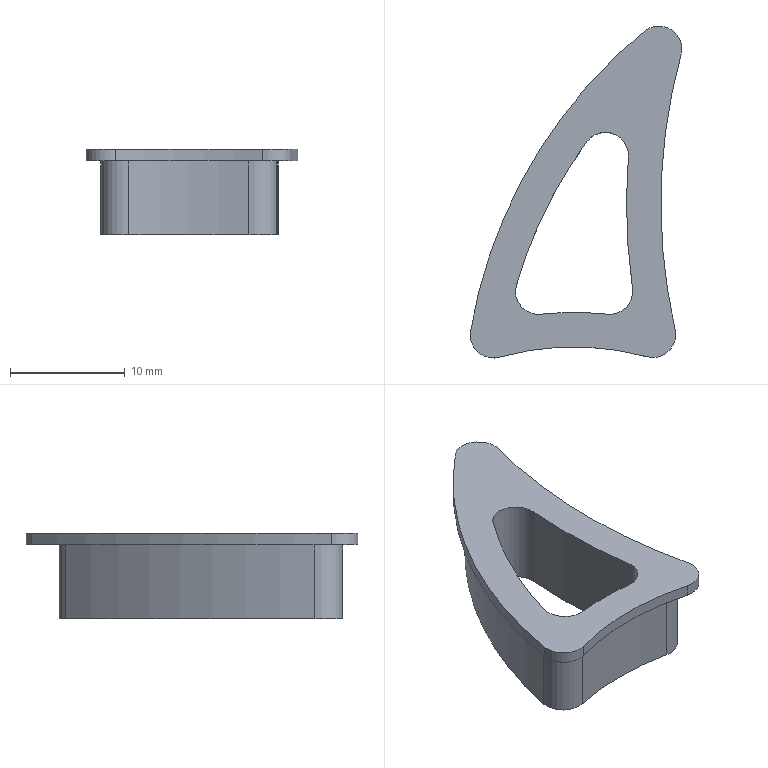Part | NX | features DATUM_CSYS 4, EXTRUDE 3, SKETCH 3, BLEND 1, CPROJ 1 | 1 solid | 21 faces | box 18.409 x 28.891 x 7.4 mm | volume 1102 mm3 | cylinder 18 | plane 3 | commonest cylinder face diameters 4 x9 48 x1 50 x1 54 x1 80 x1 84 x1
STEP:
#1=CARTESIAN_POINT('',(-5.33,24.506,0.));
#2=VERTEX_POINT('',#1);
#3=CARTESIAN_POINT('',(5.135,24.548,0.));
#4=VERTEX_POINT('',#3);
#5=CARTESIAN_POINT('',(0.,0.0809,0.));
#6=DIRECTION('',(0.,0.,-1.));
#7=DIRECTION('',(1.,0.,0.));
#8=AXIS2_PLACEMENT_3D('',#5,#6,#7);
#9=CIRCLE('',#8,25.);
#10=EDGE_CURVE('',#2,#4,#9,.T.);
#11=ORIENTED_EDGE('',*,*,#10,.F.);
#12=CARTESIAN_POINT('',(-7.715,26.867,0.));
#13=VERTEX_POINT('',#12);
#14=CARTESIAN_POINT('',(-5.757,26.46,0.));
#15=DIRECTION('',(0.,0.,-1.));
#16=DIRECTION('',(-1.,0.,0.));
#17=AXIS2_PLACEMENT_3D('',#14,#15,#16);
#18=CIRCLE('',#17,2.);
#19=EDGE_CURVE('',#2,#13,#18,.T.);
#20=ORIENTED_EDGE('',*,*,#19,.T.);
#21=CARTESIAN_POINT('',(4.276,48.579,0.));
#22=VERTEX_POINT('',#21);
#23=CARTESIAN_POINT('',(33.407,18.323,0.));
#24=DIRECTION('',(0.,0.,1.));
#25=DIRECTION('',(1.,0.,0.));
#26=AXIS2_PLACEMENT_3D('',#23,#24,#25);
#27=CIRCLE('',#26,42.);
#28=EDGE_CURVE('',#22,#13,#27,.T.);
#29=ORIENTED_EDGE('',*,*,#28,.F.);
#30=CARTESIAN_POINT('',(7.621,46.73,0.));
#31=VERTEX_POINT('',#30);
#32=CARTESIAN_POINT('',(5.663,47.138,0.));
#33=DIRECTION('',(0.,0.,-1.));
#34=DIRECTION('',(-1.,0.,0.));
#35=AXIS2_PLACEMENT_3D('',#32,#33,#34);
#36=CIRCLE('',#35,2.);
#37=EDGE_CURVE('',#22,#31,#36,.T.);
#38=ORIENTED_EDGE('',*,*,#37,.T.);
#39=CARTESIAN_POINT('',(7.509,26.891,0.));
#40=VERTEX_POINT('',#39);
#41=CARTESIAN_POINT('',(56.57,36.531,0.));
#42=DIRECTION('',(0.,0.,-1.));
#43=DIRECTION('',(1.,0.,0.));
#44=AXIS2_PLACEMENT_3D('',#41,#42,#43);
#45=CIRCLE('',#44,50.);
#46=EDGE_CURVE('',#40,#31,#45,.T.);
#47=ORIENTED_EDGE('',*,*,#46,.F.);
#48=CARTESIAN_POINT('',(5.546,26.505,0.));
#49=DIRECTION('',(0.,0.,-1.));
#50=DIRECTION('',(-1.,0.,0.));
#51=AXIS2_PLACEMENT_3D('',#48,#49,#50);
#52=CIRCLE('',#51,2.);
#53=EDGE_CURVE('',#40,#4,#52,.T.);
#54=ORIENTED_EDGE('',*,*,#53,.T.);
#55=EDGE_LOOP('',(#11,#20,#29,#38,#47,#54));
#56=FACE_BOUND('',#55,.T.);
#57=CARTESIAN_POINT('',(-2.874,26.928,0.));
#58=VERTEX_POINT('',#57);
#59=CARTESIAN_POINT('',(-5.007,29.474,0.));
#60=VERTEX_POINT('',#59);
#61=CARTESIAN_POINT('',(-3.087,28.916,0.));
#62=DIRECTION('',(0.,0.,-1.));
#63=DIRECTION('',(1.,0.,0.));
#64=AXIS2_PLACEMENT_3D('',#61,#62,#63);
#65=CIRCLE('',#64,2.);
#66=EDGE_CURVE('',#58,#60,#65,.T.);
#67=ORIENTED_EDGE('',*,*,#66,.F.);
#68=CARTESIAN_POINT('',(2.896,26.925,0.));
#69=VERTEX_POINT('',#68);
#70=CARTESIAN_POINT('',(0.,0.0809,0.));
#71=DIRECTION('',(0.,0.,1.));
#72=DIRECTION('',(1.,0.,0.));
#73=AXIS2_PLACEMENT_3D('',#70,#71,#72);
#74=CIRCLE('',#73,27.);
#75=EDGE_CURVE('',#69,#58,#74,.T.);
#76=ORIENTED_EDGE('',*,*,#75,.F.);
#77=CARTESIAN_POINT('',(5.09,29.196,0.));
#78=VERTEX_POINT('',#77);
#79=CARTESIAN_POINT('',(3.11,28.914,0.));
#80=DIRECTION('',(0.,0.,-1.));
#81=DIRECTION('',(1.,0.,0.));
#82=AXIS2_PLACEMENT_3D('',#79,#80,#81);
#83=CIRCLE('',#82,2.);
#84=EDGE_CURVE('',#78,#69,#83,.T.);
#85=ORIENTED_EDGE('',*,*,#84,.F.);
#86=CARTESIAN_POINT('',(4.73,40.6,0.));
#87=VERTEX_POINT('',#86);
#88=CARTESIAN_POINT('',(56.57,36.531,0.));
#89=DIRECTION('',(0.,0.,1.));
#90=DIRECTION('',(1.,0.,0.));
#91=AXIS2_PLACEMENT_3D('',#88,#89,#90);
#92=CIRCLE('',#91,52.);
#93=EDGE_CURVE('',#87,#78,#92,.T.);
#94=ORIENTED_EDGE('',*,*,#93,.F.);
#95=CARTESIAN_POINT('',(1.122,41.938,0.));
#96=VERTEX_POINT('',#95);
#97=CARTESIAN_POINT('',(2.736,40.757,0.));
#98=DIRECTION('',(0.,0.,-1.));
#99=DIRECTION('',(1.,0.,0.));
#100=AXIS2_PLACEMENT_3D('',#97,#98,#99);
#101=CIRCLE('',#100,2.);
#102=EDGE_CURVE('',#96,#87,#101,.T.);
#103=ORIENTED_EDGE('',*,*,#102,.F.);
#104=CARTESIAN_POINT('',(33.407,18.323,0.));
#105=DIRECTION('',(0.,0.,-1.));
#106=DIRECTION('',(1.,0.,0.));
#107=AXIS2_PLACEMENT_3D('',#104,#105,#106);
#108=CIRCLE('',#107,40.);
#109=EDGE_CURVE('',#60,#96,#108,.T.);
#110=ORIENTED_EDGE('',*,*,#109,.F.);
#111=EDGE_LOOP('',(#67,#76,#85,#94,#103,#110));
#112=FACE_BOUND('',#111,.T.);
#113=CARTESIAN_POINT('',(28.285,18.306,0.));
#114=DIRECTION('',(0.,0.,-1.));
#115=DIRECTION('',(-1.,0.,0.));
#116=AXIS2_PLACEMENT_3D('',#113,#114,#115);
#117=PLANE('',#116);
#118=ADVANCED_FACE('',(#56,#112),#117,.T.);
#119=CARTESIAN_POINT('',(-8.999,25.445,7.4));
#120=VERTEX_POINT('',#119);
#121=CARTESIAN_POINT('',(6.113,51.55,7.4));
#122=VERTEX_POINT('',#121);
#123=CARTESIAN_POINT('',(33.407,18.323,7.4));
#124=DIRECTION('',(0.,0.,1.));
#125=DIRECTION('',(1.,0.,0.));
#126=AXIS2_PLACEMENT_3D('',#123,#124,#125);
#127=CIRCLE('',#126,43.);
#128=EDGE_CURVE('',#120,#122,#127,.F.);
#129=ORIENTED_EDGE('',*,*,#128,.F.);
#130=CARTESIAN_POINT('',(-6.486,23.188,7.4));
#131=VERTEX_POINT('',#130);
#132=CARTESIAN_POINT('',(-7.027,25.113,7.4));
#133=DIRECTION('',(0.,0.,-1.));
#134=DIRECTION('',(-1.,0.,0.));
#135=AXIS2_PLACEMENT_3D('',#132,#133,#134);
#136=CIRCLE('',#135,2.);
#137=EDGE_CURVE('',#120,#131,#136,.F.);
#138=ORIENTED_EDGE('',*,*,#137,.T.);
#139=CARTESIAN_POINT('',(6.327,23.232,7.4));
#140=VERTEX_POINT('',#139);
#141=CARTESIAN_POINT('',(0.,0.0809,7.4));
#142=DIRECTION('',(0.,0.,-1.));
#143=DIRECTION('',(1.,0.,0.));
#144=AXIS2_PLACEMENT_3D('',#141,#142,#143);
#145=CIRCLE('',#144,24.);
#146=EDGE_CURVE('',#140,#131,#145,.F.);
#147=ORIENTED_EDGE('',*,*,#146,.F.);
#148=CARTESIAN_POINT('',(8.804,25.607,7.4));
#149=VERTEX_POINT('',#148);
#150=CARTESIAN_POINT('',(6.854,25.161,7.4));
#151=DIRECTION('',(0.,0.,-1.));
#152=DIRECTION('',(-1.,0.,0.));
#153=AXIS2_PLACEMENT_3D('',#150,#151,#152);
#154=CIRCLE('',#153,2.);
#155=EDGE_CURVE('',#140,#149,#154,.F.);
#156=ORIENTED_EDGE('',*,*,#155,.T.);
#157=CARTESIAN_POINT('',(9.311,49.476,7.4));
#158=VERTEX_POINT('',#157);
#159=CARTESIAN_POINT('',(56.57,36.531,7.4));
#160=DIRECTION('',(0.,0.,-1.));
#161=DIRECTION('',(1.,0.,0.));
#162=AXIS2_PLACEMENT_3D('',#159,#160,#161);
#163=CIRCLE('',#162,49.);
#164=EDGE_CURVE('',#158,#149,#163,.F.);
#165=ORIENTED_EDGE('',*,*,#164,.F.);
#166=CARTESIAN_POINT('',(7.382,50.004,7.4));
#167=DIRECTION('',(0.,0.,-1.));
#168=DIRECTION('',(-1.,0.,0.));
#169=AXIS2_PLACEMENT_3D('',#166,#167,#168);
#170=CIRCLE('',#169,2.);
#171=EDGE_CURVE('',#158,#122,#170,.F.);
#172=ORIENTED_EDGE('',*,*,#171,.T.);
#173=EDGE_LOOP('',(#129,#138,#147,#156,#165,#172));
#174=FACE_BOUND('',#173,.T.);
#175=CARTESIAN_POINT('',(2.896,26.925,7.4));
#176=VERTEX_POINT('',#175);
#177=CARTESIAN_POINT('',(-2.874,26.928,7.4));
#178=VERTEX_POINT('',#177);
#179=CARTESIAN_POINT('',(0.,0.0809,7.4));
#180=DIRECTION('',(0.,0.,-1.));
#181=DIRECTION('',(-1.,0.,0.));
#182=AXIS2_PLACEMENT_3D('',#179,#180,#181);
#183=CIRCLE('',#182,27.);
#184=EDGE_CURVE('',#176,#178,#183,.F.);
#185=ORIENTED_EDGE('',*,*,#184,.T.);
#186=CARTESIAN_POINT('',(-5.007,29.474,7.4));
#187=VERTEX_POINT('',#186);
#188=CARTESIAN_POINT('',(-3.087,28.916,7.4));
#189=DIRECTION('',(0.,0.,-1.));
#190=DIRECTION('',(-1.,0.,0.));
#191=AXIS2_PLACEMENT_3D('',#188,#189,#190);
#192=CIRCLE('',#191,2.);
#193=EDGE_CURVE('',#178,#187,#192,.T.);
#194=ORIENTED_EDGE('',*,*,#193,.T.);
#195=CARTESIAN_POINT('',(1.122,41.938,7.4));
#196=VERTEX_POINT('',#195);
#197=CARTESIAN_POINT('',(33.407,18.323,7.4));
#198=DIRECTION('',(0.,0.,-1.));
#199=DIRECTION('',(-1.,0.,0.));
#200=AXIS2_PLACEMENT_3D('',#197,#198,#199);
#201=CIRCLE('',#200,40.);
#202=EDGE_CURVE('',#187,#196,#201,.T.);
#203=ORIENTED_EDGE('',*,*,#202,.T.);
#204=CARTESIAN_POINT('',(4.73,40.6,7.4));
#205=VERTEX_POINT('',#204);
#206=CARTESIAN_POINT('',(2.736,40.757,7.4));
#207=DIRECTION('',(0.,0.,-1.));
#208=DIRECTION('',(-1.,0.,0.));
#209=AXIS2_PLACEMENT_3D('',#206,#207,#208);
#210=CIRCLE('',#209,2.);
#211=EDGE_CURVE('',#196,#205,#210,.T.);
#212=ORIENTED_EDGE('',*,*,#211,.T.);
#213=CARTESIAN_POINT('',(5.09,29.196,7.4));
#214=VERTEX_POINT('',#213);
#215=CARTESIAN_POINT('',(56.57,36.531,7.4));
#216=DIRECTION('',(0.,0.,-1.));
#217=DIRECTION('',(-1.,0.,0.));
#218=AXIS2_PLACEMENT_3D('',#215,#216,#217);
#219=CIRCLE('',#218,52.);
#220=EDGE_CURVE('',#205,#214,#219,.F.);
#221=ORIENTED_EDGE('',*,*,#220,.T.);
#222=CARTESIAN_POINT('',(3.11,28.914,7.4));
#223=DIRECTION('',(0.,0.,-1.));
#224=DIRECTION('',(-1.,0.,0.));
#225=AXIS2_PLACEMENT_3D('',#222,#223,#224);
#226=CIRCLE('',#225,2.);
#227=EDGE_CURVE('',#214,#176,#226,.T.);
#228=ORIENTED_EDGE('',*,*,#227,.T.);
#229=EDGE_LOOP('',(#185,#194,#203,#212,#221,#228));
#230=FACE_BOUND('',#229,.T.);
#231=CARTESIAN_POINT('',(28.285,18.306,7.4));
#232=DIRECTION('',(0.,0.,-1.));
#233=DIRECTION('',(-1.,0.,0.));
#234=AXIS2_PLACEMENT_3D('',#231,#232,#233);
#235=PLANE('',#234);
#236=ADVANCED_FACE('',(#174,#230),#235,.F.);
#237=CARTESIAN_POINT('',(-5.33,24.506,6.4));
#238=VERTEX_POINT('',#237);
#239=CARTESIAN_POINT('',(5.135,24.548,6.4));
#240=VERTEX_POINT('',#239);
#241=CARTESIAN_POINT('',(0.,0.0809,6.4));
#242=DIRECTION('',(0.,0.,1.));
#243=DIRECTION('',(1.,0.,0.));
#244=AXIS2_PLACEMENT_3D('',#241,#242,#243);
#245=CIRCLE('',#244,25.);
#246=EDGE_CURVE('',#238,#240,#245,.F.);
#247=ORIENTED_EDGE('',*,*,#246,.F.);
#248=CARTESIAN_POINT('',(-5.33,24.506,7.4));
#249=DIRECTION('',(0.,0.,-1.));
#250=VECTOR('',#249,1000.);
#251=LINE('',#248,#250);
#252=EDGE_CURVE('',#238,#2,#251,.T.);
#253=ORIENTED_EDGE('',*,*,#252,.T.);
#254=ORIENTED_EDGE('',*,*,#10,.T.);
#255=CARTESIAN_POINT('',(5.135,24.548,7.4));
#256=DIRECTION('',(0.,0.,-1.));
#257=VECTOR('',#256,1000.);
#258=LINE('',#255,#257);
#259=EDGE_CURVE('',#4,#240,#258,.F.);
#260=ORIENTED_EDGE('',*,*,#259,.T.);
#261=EDGE_LOOP('',(#247,#253,#254,#260));
#262=FACE_BOUND('',#261,.T.);
#263=CARTESIAN_POINT('',(0.,0.0809,7.4));
#264=DIRECTION('',(0.,0.,-1.));
#265=DIRECTION('',(-1.,0.,0.));
#266=AXIS2_PLACEMENT_3D('',#263,#264,#265);
#267=CYLINDRICAL_SURFACE('',#266,25.);
#268=ADVANCED_FACE('',(#262),#267,.F.);
#269=CARTESIAN_POINT('',(7.509,26.891,6.4));
#270=VERTEX_POINT('',#269);
#271=CARTESIAN_POINT('',(7.621,46.73,6.4));
#272=VERTEX_POINT('',#271);
#273=CARTESIAN_POINT('',(56.57,36.531,6.4));
#274=DIRECTION('',(0.,0.,1.));
#275=DIRECTION('',(1.,0.,0.));
#276=AXIS2_PLACEMENT_3D('',#273,#274,#275);
#277=CIRCLE('',#276,50.);
#278=EDGE_CURVE('',#270,#272,#277,.F.);
#279=ORIENTED_EDGE('',*,*,#278,.F.);
#280=CARTESIAN_POINT('',(7.509,26.891,7.4));
#281=DIRECTION('',(0.,0.,-1.));
#282=VECTOR('',#281,1000.);
#283=LINE('',#280,#282);
#284=EDGE_CURVE('',#270,#40,#283,.T.);
#285=ORIENTED_EDGE('',*,*,#284,.T.);
#286=ORIENTED_EDGE('',*,*,#46,.T.);
#287=CARTESIAN_POINT('',(7.621,46.73,7.4));
#288=DIRECTION('',(0.,0.,-1.));
#289=VECTOR('',#288,1000.);
#290=LINE('',#287,#289);
#291=EDGE_CURVE('',#31,#272,#290,.F.);
#292=ORIENTED_EDGE('',*,*,#291,.T.);
#293=EDGE_LOOP('',(#279,#285,#286,#292));
#294=FACE_BOUND('',#293,.T.);
#295=CARTESIAN_POINT('',(56.57,36.531,7.4));
#296=DIRECTION('',(0.,0.,-1.));
#297=DIRECTION('',(-1.,0.,0.));
#298=AXIS2_PLACEMENT_3D('',#295,#296,#297);
#299=CYLINDRICAL_SURFACE('',#298,50.);
#300=ADVANCED_FACE('',(#294),#299,.F.);
#301=ORIENTED_EDGE('',*,*,#28,.T.);
#302=CARTESIAN_POINT('',(-7.715,26.867,6.4));
#303=VERTEX_POINT('',#302);
#304=CARTESIAN_POINT('',(-7.715,26.867,7.4));
#305=DIRECTION('',(0.,0.,-1.));
#306=VECTOR('',#305,1000.);
#307=LINE('',#304,#306);
#308=EDGE_CURVE('',#13,#303,#307,.F.);
#309=ORIENTED_EDGE('',*,*,#308,.T.);
#310=CARTESIAN_POINT('',(4.276,48.579,6.4));
#311=VERTEX_POINT('',#310);
#312=CARTESIAN_POINT('',(33.407,18.323,6.4));
#313=DIRECTION('',(0.,0.,-1.));
#314=DIRECTION('',(1.,0.,0.));
#315=AXIS2_PLACEMENT_3D('',#312,#313,#314);
#316=CIRCLE('',#315,42.);
#317=EDGE_CURVE('',#311,#303,#316,.F.);
#318=ORIENTED_EDGE('',*,*,#317,.F.);
#319=CARTESIAN_POINT('',(4.276,48.579,7.4));
#320=DIRECTION('',(0.,0.,-1.));
#321=VECTOR('',#320,1000.);
#322=LINE('',#319,#321);
#323=EDGE_CURVE('',#311,#22,#322,.T.);
#324=ORIENTED_EDGE('',*,*,#323,.T.);
#325=EDGE_LOOP('',(#301,#309,#318,#324));
#326=FACE_BOUND('',#325,.T.);
#327=CARTESIAN_POINT('',(33.407,18.323,7.4));
#328=DIRECTION('',(0.,0.,-1.));
#329=DIRECTION('',(-1.,0.,0.));
#330=AXIS2_PLACEMENT_3D('',#327,#328,#329);
#331=CYLINDRICAL_SURFACE('',#330,42.);
#332=ADVANCED_FACE('',(#326),#331,.T.);
#333=ORIENTED_EDGE('',*,*,#146,.T.);
#334=CARTESIAN_POINT('',(-6.486,23.188,6.4));
#335=VERTEX_POINT('',#334);
#336=CARTESIAN_POINT('',(-6.486,23.188,6.4));
#337=DIRECTION('',(0.,0.,1.));
#338=VECTOR('',#337,1000.);
#339=LINE('',#336,#338);
#340=EDGE_CURVE('',#131,#335,#339,.F.);
#341=ORIENTED_EDGE('',*,*,#340,.T.);
#342=CARTESIAN_POINT('',(6.327,23.232,6.4));
#343=VERTEX_POINT('',#342);
#344=CARTESIAN_POINT('',(0.,0.0809,6.4));
#345=DIRECTION('',(0.,0.,-1.));
#346=DIRECTION('',(1.,0.,0.));
#347=AXIS2_PLACEMENT_3D('',#344,#345,#346);
#348=CIRCLE('',#347,24.);
#349=EDGE_CURVE('',#343,#335,#348,.F.);
#350=ORIENTED_EDGE('',*,*,#349,.F.);
#351=CARTESIAN_POINT('',(6.327,23.232,6.4));
#352=DIRECTION('',(0.,0.,1.));
#353=VECTOR('',#352,1000.);
#354=LINE('',#351,#353);
#355=EDGE_CURVE('',#343,#140,#354,.T.);
#356=ORIENTED_EDGE('',*,*,#355,.T.);
#357=EDGE_LOOP('',(#333,#341,#350,#356));
#358=FACE_BOUND('',#357,.T.);
#359=CARTESIAN_POINT('',(0.,0.0809,6.4));
#360=DIRECTION('',(0.,0.,1.));
#361=DIRECTION('',(1.,0.,0.));
#362=AXIS2_PLACEMENT_3D('',#359,#360,#361);
#363=CYLINDRICAL_SURFACE('',#362,24.);
#364=ADVANCED_FACE('',(#358),#363,.F.);
#365=ORIENTED_EDGE('',*,*,#164,.T.);
#366=CARTESIAN_POINT('',(8.804,25.607,6.4));
#367=VERTEX_POINT('',#366);
#368=CARTESIAN_POINT('',(8.804,25.607,6.4));
#369=DIRECTION('',(0.,0.,1.));
#370=VECTOR('',#369,1000.);
#371=LINE('',#368,#370);
#372=EDGE_CURVE('',#149,#367,#371,.F.);
#373=ORIENTED_EDGE('',*,*,#372,.T.);
#374=CARTESIAN_POINT('',(9.311,49.476,6.4));
#375=VERTEX_POINT('',#374);
#376=CARTESIAN_POINT('',(56.57,36.531,6.4));
#377=DIRECTION('',(0.,0.,-1.));
#378=DIRECTION('',(1.,0.,0.));
#379=AXIS2_PLACEMENT_3D('',#376,#377,#378);
#380=CIRCLE('',#379,49.);
#381=EDGE_CURVE('',#375,#367,#380,.F.);
#382=ORIENTED_EDGE('',*,*,#381,.F.);
#383=CARTESIAN_POINT('',(9.311,49.476,6.4));
#384=DIRECTION('',(0.,0.,1.));
#385=VECTOR('',#384,1000.);
#386=LINE('',#383,#385);
#387=EDGE_CURVE('',#375,#158,#386,.T.);
#388=ORIENTED_EDGE('',*,*,#387,.T.);
#389=EDGE_LOOP('',(#365,#373,#382,#388));
#390=FACE_BOUND('',#389,.T.);
#391=CARTESIAN_POINT('',(56.57,36.531,6.4));
#392=DIRECTION('',(0.,0.,1.));
#393=DIRECTION('',(1.,0.,0.));
#394=AXIS2_PLACEMENT_3D('',#391,#392,#393);
#395=CYLINDRICAL_SURFACE('',#394,49.);
#396=ADVANCED_FACE('',(#390),#395,.F.);
#397=CARTESIAN_POINT('',(-8.999,25.445,6.4));
#398=VERTEX_POINT('',#397);
#399=CARTESIAN_POINT('',(6.113,51.55,6.4));
#400=VERTEX_POINT('',#399);
#401=CARTESIAN_POINT('',(33.407,18.323,6.4));
#402=DIRECTION('',(0.,0.,1.));
#403=DIRECTION('',(1.,0.,0.));
#404=AXIS2_PLACEMENT_3D('',#401,#402,#403);
#405=CIRCLE('',#404,43.);
#406=EDGE_CURVE('',#398,#400,#405,.F.);
#407=ORIENTED_EDGE('',*,*,#406,.F.);
#408=CARTESIAN_POINT('',(-8.999,25.445,6.4));
#409=DIRECTION('',(0.,0.,1.));
#410=VECTOR('',#409,1000.);
#411=LINE('',#408,#410);
#412=EDGE_CURVE('',#398,#120,#411,.T.);
#413=ORIENTED_EDGE('',*,*,#412,.T.);
#414=ORIENTED_EDGE('',*,*,#128,.T.);
#415=CARTESIAN_POINT('',(6.113,51.55,6.4));
#416=DIRECTION('',(0.,0.,1.));
#417=VECTOR('',#416,1000.);
#418=LINE('',#415,#417);
#419=EDGE_CURVE('',#122,#400,#418,.F.);
#420=ORIENTED_EDGE('',*,*,#419,.T.);
#421=EDGE_LOOP('',(#407,#413,#414,#420));
#422=FACE_BOUND('',#421,.T.);
#423=CARTESIAN_POINT('',(33.407,18.323,6.4));
#424=DIRECTION('',(0.,0.,1.));
#425=DIRECTION('',(1.,0.,0.));
#426=AXIS2_PLACEMENT_3D('',#423,#424,#425);
#427=CYLINDRICAL_SURFACE('',#426,43.);
#428=ADVANCED_FACE('',(#422),#427,.T.);
#429=ORIENTED_EDGE('',*,*,#381,.T.);
#430=CARTESIAN_POINT('',(6.854,25.161,6.4));
#431=DIRECTION('',(0.,0.,-1.));
#432=DIRECTION('',(-1.,0.,0.));
#433=AXIS2_PLACEMENT_3D('',#430,#431,#432);
#434=CIRCLE('',#433,2.);
#435=EDGE_CURVE('',#367,#343,#434,.T.);
#436=ORIENTED_EDGE('',*,*,#435,.T.);
#437=ORIENTED_EDGE('',*,*,#349,.T.);
#438=CARTESIAN_POINT('',(-7.027,25.113,6.4));
#439=DIRECTION('',(0.,0.,-1.));
#440=DIRECTION('',(-1.,0.,0.));
#441=AXIS2_PLACEMENT_3D('',#438,#439,#440);
#442=CIRCLE('',#441,2.);
#443=EDGE_CURVE('',#335,#398,#442,.T.);
#444=ORIENTED_EDGE('',*,*,#443,.T.);
#445=ORIENTED_EDGE('',*,*,#406,.T.);
#446=CARTESIAN_POINT('',(7.382,50.004,6.4));
#447=DIRECTION('',(0.,0.,-1.));
#448=DIRECTION('',(-1.,0.,0.));
#449=AXIS2_PLACEMENT_3D('',#446,#447,#448);
#450=CIRCLE('',#449,2.);
#451=EDGE_CURVE('',#400,#375,#450,.T.);
#452=ORIENTED_EDGE('',*,*,#451,.T.);
#453=EDGE_LOOP('',(#429,#436,#437,#444,#445,#452));
#454=FACE_BOUND('',#453,.T.);
#455=ORIENTED_EDGE('',*,*,#317,.T.);
#456=CARTESIAN_POINT('',(-5.757,26.46,6.4));
#457=DIRECTION('',(0.,0.,-1.));
#458=DIRECTION('',(-1.,0.,0.));
#459=AXIS2_PLACEMENT_3D('',#456,#457,#458);
#460=CIRCLE('',#459,2.);
#461=EDGE_CURVE('',#303,#238,#460,.F.);
#462=ORIENTED_EDGE('',*,*,#461,.T.);
#463=ORIENTED_EDGE('',*,*,#246,.T.);
#464=CARTESIAN_POINT('',(5.546,26.505,6.4));
#465=DIRECTION('',(0.,0.,-1.));
#466=DIRECTION('',(-1.,0.,0.));
#467=AXIS2_PLACEMENT_3D('',#464,#465,#466);
#468=CIRCLE('',#467,2.);
#469=EDGE_CURVE('',#240,#270,#468,.F.);
#470=ORIENTED_EDGE('',*,*,#469,.T.);
#471=ORIENTED_EDGE('',*,*,#278,.T.);
#472=CARTESIAN_POINT('',(5.663,47.138,6.4));
#473=DIRECTION('',(0.,0.,-1.));
#474=DIRECTION('',(-1.,0.,0.));
#475=AXIS2_PLACEMENT_3D('',#472,#473,#474);
#476=CIRCLE('',#475,2.);
#477=EDGE_CURVE('',#272,#311,#476,.F.);
#478=ORIENTED_EDGE('',*,*,#477,.T.);
#479=EDGE_LOOP('',(#455,#462,#463,#470,#471,#478));
#480=FACE_BOUND('',#479,.T.);
#481=CARTESIAN_POINT('',(28.285,18.306,6.4));
#482=DIRECTION('',(0.,0.,-1.));
#483=DIRECTION('',(-1.,0.,0.));
#484=AXIS2_PLACEMENT_3D('',#481,#482,#483);
#485=PLANE('',#484);
#486=ADVANCED_FACE('',(#454,#480),#485,.T.);
#487=CARTESIAN_POINT('',(-2.874,26.928,55000.));
#488=DIRECTION('',(0.,0.,-1.));
#489=VECTOR('',#488,1000.);
#490=LINE('',#487,#489);
#491=EDGE_CURVE('',#58,#178,#490,.F.);
#492=ORIENTED_EDGE('',*,*,#491,.F.);
#493=ORIENTED_EDGE('',*,*,#66,.T.);
#494=CARTESIAN_POINT('',(-5.007,29.474,55000.));
#495=DIRECTION('',(0.,0.,-1.));
#496=VECTOR('',#495,1000.);
#497=LINE('',#494,#496);
#498=EDGE_CURVE('',#60,#187,#497,.F.);
#499=ORIENTED_EDGE('',*,*,#498,.T.);
#500=ORIENTED_EDGE('',*,*,#193,.F.);
#501=EDGE_LOOP('',(#492,#493,#499,#500));
#502=FACE_BOUND('',#501,.T.);
#503=CARTESIAN_POINT('',(-3.087,28.916,55000.));
#504=DIRECTION('',(0.,0.,-1.));
#505=DIRECTION('',(-1.,0.,0.));
#506=AXIS2_PLACEMENT_3D('',#503,#504,#505);
#507=CYLINDRICAL_SURFACE('',#506,2.);
#508=ADVANCED_FACE('',(#502),#507,.F.);
#509=ORIENTED_EDGE('',*,*,#498,.F.);
#510=ORIENTED_EDGE('',*,*,#109,.T.);
#511=CARTESIAN_POINT('',(1.122,41.938,55000.));
#512=DIRECTION('',(0.,0.,-1.));
#513=VECTOR('',#512,1000.);
#514=LINE('',#511,#513);
#515=EDGE_CURVE('',#96,#196,#514,.F.);
#516=ORIENTED_EDGE('',*,*,#515,.T.);
#517=ORIENTED_EDGE('',*,*,#202,.F.);
#518=EDGE_LOOP('',(#509,#510,#516,#517));
#519=FACE_BOUND('',#518,.T.);
#520=CARTESIAN_POINT('',(33.407,18.323,55000.));
#521=DIRECTION('',(0.,0.,-1.));
#522=DIRECTION('',(-1.,0.,0.));
#523=AXIS2_PLACEMENT_3D('',#520,#521,#522);
#524=CYLINDRICAL_SURFACE('',#523,40.);
#525=ADVANCED_FACE('',(#519),#524,.F.);
#526=ORIENTED_EDGE('',*,*,#515,.F.);
#527=ORIENTED_EDGE('',*,*,#102,.T.);
#528=CARTESIAN_POINT('',(4.73,40.6,55000.));
#529=DIRECTION('',(0.,0.,-1.));
#530=VECTOR('',#529,1000.);
#531=LINE('',#528,#530);
#532=EDGE_CURVE('',#87,#205,#531,.F.);
#533=ORIENTED_EDGE('',*,*,#532,.T.);
#534=ORIENTED_EDGE('',*,*,#211,.F.);
#535=EDGE_LOOP('',(#526,#527,#533,#534));
#536=FACE_BOUND('',#535,.T.);
#537=CARTESIAN_POINT('',(2.736,40.757,55000.));
#538=DIRECTION('',(0.,0.,-1.));
#539=DIRECTION('',(-1.,0.,0.));
#540=AXIS2_PLACEMENT_3D('',#537,#538,#539);
#541=CYLINDRICAL_SURFACE('',#540,2.);
#542=ADVANCED_FACE('',(#536),#541,.F.);
#543=ORIENTED_EDGE('',*,*,#532,.F.);
#544=ORIENTED_EDGE('',*,*,#93,.T.);
#545=CARTESIAN_POINT('',(5.09,29.196,55000.));
#546=DIRECTION('',(0.,0.,-1.));
#547=VECTOR('',#546,1000.);
#548=LINE('',#545,#547);
#549=EDGE_CURVE('',#78,#214,#548,.F.);
#550=ORIENTED_EDGE('',*,*,#549,.T.);
#551=ORIENTED_EDGE('',*,*,#220,.F.);
#552=EDGE_LOOP('',(#543,#544,#550,#551));
#553=FACE_BOUND('',#552,.T.);
#554=CARTESIAN_POINT('',(56.57,36.531,55000.));
#555=DIRECTION('',(0.,0.,-1.));
#556=DIRECTION('',(-1.,0.,0.));
#557=AXIS2_PLACEMENT_3D('',#554,#555,#556);
#558=CYLINDRICAL_SURFACE('',#557,52.);
#559=ADVANCED_FACE('',(#553),#558,.T.);
#560=ORIENTED_EDGE('',*,*,#549,.F.);
#561=ORIENTED_EDGE('',*,*,#84,.T.);
#562=CARTESIAN_POINT('',(2.896,26.925,55000.));
#563=DIRECTION('',(0.,0.,-1.));
#564=VECTOR('',#563,1000.);
#565=LINE('',#562,#564);
#566=EDGE_CURVE('',#69,#176,#565,.F.);
#567=ORIENTED_EDGE('',*,*,#566,.T.);
#568=ORIENTED_EDGE('',*,*,#227,.F.);
#569=EDGE_LOOP('',(#560,#561,#567,#568));
#570=FACE_BOUND('',#569,.T.);
#571=CARTESIAN_POINT('',(3.11,28.914,55000.));
#572=DIRECTION('',(0.,0.,-1.));
#573=DIRECTION('',(-1.,0.,0.));
#574=AXIS2_PLACEMENT_3D('',#571,#572,#573);
#575=CYLINDRICAL_SURFACE('',#574,2.);
#576=ADVANCED_FACE('',(#570),#575,.F.);
#577=ORIENTED_EDGE('',*,*,#566,.F.);
#578=ORIENTED_EDGE('',*,*,#75,.T.);
#579=ORIENTED_EDGE('',*,*,#491,.T.);
#580=ORIENTED_EDGE('',*,*,#184,.F.);
#581=EDGE_LOOP('',(#577,#578,#579,#580));
#582=FACE_BOUND('',#581,.T.);
#583=CARTESIAN_POINT('',(0.,0.0809,55000.));
#584=DIRECTION('',(0.,0.,-1.));
#585=DIRECTION('',(-1.,0.,0.));
#586=AXIS2_PLACEMENT_3D('',#583,#584,#585);
#587=CYLINDRICAL_SURFACE('',#586,27.);
#588=ADVANCED_FACE('',(#582),#587,.T.);
#589=ORIENTED_EDGE('',*,*,#137,.F.);
#590=ORIENTED_EDGE('',*,*,#412,.F.);
#591=ORIENTED_EDGE('',*,*,#443,.F.);
#592=ORIENTED_EDGE('',*,*,#340,.F.);
#593=EDGE_LOOP('',(#589,#590,#591,#592));
#594=FACE_BOUND('',#593,.T.);
#595=CARTESIAN_POINT('',(-7.027,25.113,6.4));
#596=DIRECTION('',(0.,0.,1.));
#597=DIRECTION('',(1.,0.,0.));
#598=AXIS2_PLACEMENT_3D('',#595,#596,#597);
#599=CYLINDRICAL_SURFACE('',#598,2.);
#600=ADVANCED_FACE('',(#594),#599,.T.);
#601=ORIENTED_EDGE('',*,*,#155,.F.);
#602=ORIENTED_EDGE('',*,*,#355,.F.);
#603=ORIENTED_EDGE('',*,*,#435,.F.);
#604=ORIENTED_EDGE('',*,*,#372,.F.);
#605=EDGE_LOOP('',(#601,#602,#603,#604));
#606=FACE_BOUND('',#605,.T.);
#607=CARTESIAN_POINT('',(6.854,25.161,6.4));
#608=DIRECTION('',(0.,0.,-1.));
#609=DIRECTION('',(-1.,0.,0.));
#610=AXIS2_PLACEMENT_3D('',#607,#608,#609);
#611=CYLINDRICAL_SURFACE('',#610,2.);
#612=ADVANCED_FACE('',(#606),#611,.T.);
#613=ORIENTED_EDGE('',*,*,#171,.F.);
#614=ORIENTED_EDGE('',*,*,#387,.F.);
#615=ORIENTED_EDGE('',*,*,#451,.F.);
#616=ORIENTED_EDGE('',*,*,#419,.F.);
#617=EDGE_LOOP('',(#613,#614,#615,#616));
#618=FACE_BOUND('',#617,.T.);
#619=CARTESIAN_POINT('',(7.382,50.004,6.4));
#620=DIRECTION('',(0.,0.,1.));
#621=DIRECTION('',(1.,0.,0.));
#622=AXIS2_PLACEMENT_3D('',#619,#620,#621);
#623=CYLINDRICAL_SURFACE('',#622,2.);
#624=ADVANCED_FACE('',(#618),#623,.T.);
#625=ORIENTED_EDGE('',*,*,#461,.F.);
#626=ORIENTED_EDGE('',*,*,#308,.F.);
#627=ORIENTED_EDGE('',*,*,#19,.F.);
#628=ORIENTED_EDGE('',*,*,#252,.F.);
#629=EDGE_LOOP('',(#625,#626,#627,#628));
#630=FACE_BOUND('',#629,.T.);
#631=CARTESIAN_POINT('',(-5.757,26.46,7.4));
#632=DIRECTION('',(0.,0.,1.));
#633=DIRECTION('',(1.,0.,0.));
#634=AXIS2_PLACEMENT_3D('',#631,#632,#633);
#635=CYLINDRICAL_SURFACE('',#634,2.);
#636=ADVANCED_FACE('',(#630),#635,.T.);
#637=ORIENTED_EDGE('',*,*,#469,.F.);
#638=ORIENTED_EDGE('',*,*,#259,.F.);
#639=ORIENTED_EDGE('',*,*,#53,.F.);
#640=ORIENTED_EDGE('',*,*,#284,.F.);
#641=EDGE_LOOP('',(#637,#638,#639,#640));
#642=FACE_BOUND('',#641,.T.);
#643=CARTESIAN_POINT('',(5.546,26.505,7.4));
#644=DIRECTION('',(0.,0.,-1.));
#645=DIRECTION('',(-1.,0.,0.));
#646=AXIS2_PLACEMENT_3D('',#643,#644,#645);
#647=CYLINDRICAL_SURFACE('',#646,2.);
#648=ADVANCED_FACE('',(#642),#647,.T.);
#649=ORIENTED_EDGE('',*,*,#477,.F.);
#650=ORIENTED_EDGE('',*,*,#291,.F.);
#651=ORIENTED_EDGE('',*,*,#37,.F.);
#652=ORIENTED_EDGE('',*,*,#323,.F.);
#653=EDGE_LOOP('',(#649,#650,#651,#652));
#654=FACE_BOUND('',#653,.T.);
#655=CARTESIAN_POINT('',(5.663,47.138,7.4));
#656=DIRECTION('',(0.,0.,1.));
#657=DIRECTION('',(1.,0.,0.));
#658=AXIS2_PLACEMENT_3D('',#655,#656,#657);
#659=CYLINDRICAL_SURFACE('',#658,2.);
#660=ADVANCED_FACE('',(#654),#659,.T.);
#661=CLOSED_SHELL('',(#118,#236,#268,#300,#332,#364,#396,#428,#486,#508,#525,#542,#559,#576,#588,#600,#612,#624,#636,#648,#660));
#662=MANIFOLD_SOLID_BREP('',#661);
#663=(LENGTH_UNIT()NAMED_UNIT(*)SI_UNIT(.MILLI.,.METRE.));
#664=UNCERTAINTY_MEASURE_WITH_UNIT(LENGTH_MEASURE(0.00001),#663,'','');
#665=(NAMED_UNIT(*)PLANE_ANGLE_UNIT()SI_UNIT($,.RADIAN.));
#666=(NAMED_UNIT(*)SI_UNIT($,.STERADIAN.)SOLID_ANGLE_UNIT());
#667=(GEOMETRIC_REPRESENTATION_CONTEXT(3)GLOBAL_UNCERTAINTY_ASSIGNED_CONTEXT((#664))GLOBAL_UNIT_ASSIGNED_CONTEXT((#663,#665,#666))REPRESENTATION_CONTEXT('',''));
#668=ADVANCED_BREP_SHAPE_REPRESENTATION('',(#662),#667);